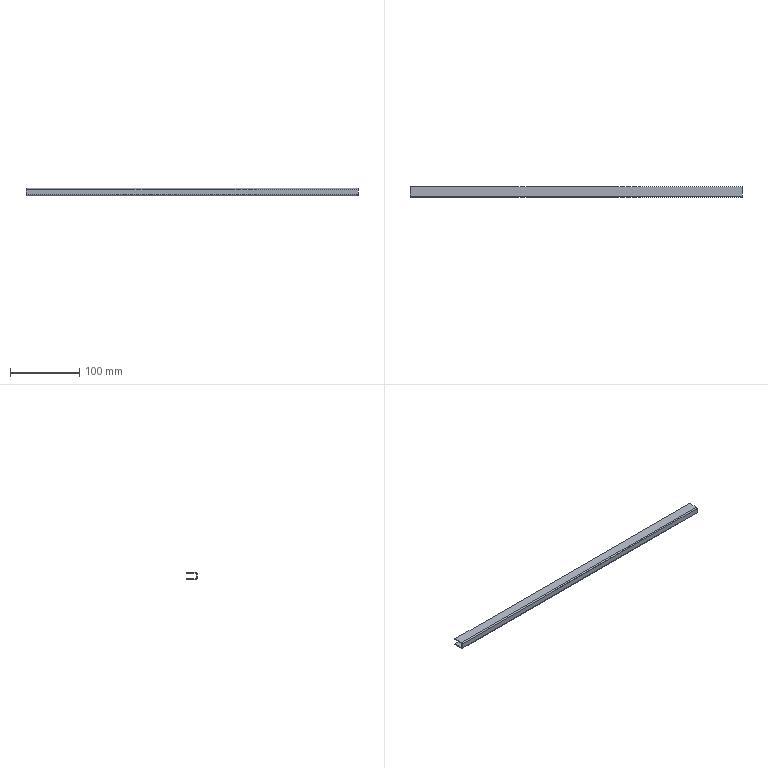Part | SolidWorks | features EdgeFlange 1, FlatPattern 1, SMBaseFlange 1, SheetMetal 1 | 1 solid | 22 faces | box 480 x 15 x 10.4 mm | volume 21369 mm3 | plane 18 | cylinder 4 | commonest cylinder face diameters 0.9 x2 3.3 x2
STEP:
#1=CARTESIAN_POINT('',(-74.374,1.2,10.26));
#2=VERTEX_POINT('',#1);
#3=CARTESIAN_POINT('',(-74.374,0.,10.26));
#4=VERTEX_POINT('',#3);
#5=CARTESIAN_POINT('',(-74.374,1.2,10.26));
#6=DIRECTION('',(0.,-1.,0.));
#7=VECTOR('',#6,1000.);
#8=LINE('',#5,#7);
#9=EDGE_CURVE('',#2,#4,#8,.T.);
#10=ORIENTED_EDGE('',*,*,#9,.F.);
#11=CARTESIAN_POINT('',(-74.374,1.2,3.16));
#12=VERTEX_POINT('',#11);
#13=CARTESIAN_POINT('',(-74.374,1.2,1.51));
#14=DIRECTION('',(0.,0.,1.));
#15=VECTOR('',#14,1000.);
#16=LINE('',#13,#15);
#17=EDGE_CURVE('',#12,#2,#16,.T.);
#18=ORIENTED_EDGE('',*,*,#17,.F.);
#19=CARTESIAN_POINT('',(-74.374,0.,3.16));
#20=VERTEX_POINT('',#19);
#21=CARTESIAN_POINT('',(-74.374,1.2,3.16));
#22=DIRECTION('',(0.,-1.,0.));
#23=VECTOR('',#22,1000.);
#24=LINE('',#21,#23);
#25=EDGE_CURVE('',#12,#20,#24,.T.);
#26=ORIENTED_EDGE('',*,*,#25,.T.);
#27=CARTESIAN_POINT('',(-74.374,0.,1.51));
#28=DIRECTION('',(0.,0.,1.));
#29=VECTOR('',#28,1000.);
#30=LINE('',#27,#29);
#31=EDGE_CURVE('',#20,#4,#30,.T.);
#32=ORIENTED_EDGE('',*,*,#31,.T.);
#33=EDGE_LOOP('',(#10,#18,#26,#32));
#34=FACE_OUTER_BOUND('',#33,.T.);
#35=CARTESIAN_POINT('',(-74.374,1.2,1.51));
#36=DIRECTION('',(1.,0.,0.));
#37=DIRECTION('',(0.,0.,-1.));
#38=AXIS2_PLACEMENT_3D('',#35,#36,#37);
#39=PLANE('',#38);
#40=ADVANCED_FACE('',(#34),#39,.F.);
#41=CARTESIAN_POINT('',(405.626,1.2,10.26));
#42=VERTEX_POINT('',#41);
#43=CARTESIAN_POINT('',(405.626,0.,10.26));
#44=VERTEX_POINT('',#43);
#45=CARTESIAN_POINT('',(405.626,1.2,10.26));
#46=DIRECTION('',(0.,-1.,0.));
#47=VECTOR('',#46,1000.);
#48=LINE('',#45,#47);
#49=EDGE_CURVE('',#42,#44,#48,.T.);
#50=ORIENTED_EDGE('',*,*,#49,.T.);
#51=CARTESIAN_POINT('',(405.626,0.,3.16));
#52=VERTEX_POINT('',#51);
#53=CARTESIAN_POINT('',(405.626,0.,1.51));
#54=DIRECTION('',(0.,0.,-1.));
#55=VECTOR('',#54,1000.);
#56=LINE('',#53,#55);
#57=EDGE_CURVE('',#44,#52,#56,.T.);
#58=ORIENTED_EDGE('',*,*,#57,.T.);
#59=CARTESIAN_POINT('',(405.626,1.2,3.16));
#60=VERTEX_POINT('',#59);
#61=CARTESIAN_POINT('',(405.626,1.2,3.16));
#62=DIRECTION('',(0.,-1.,0.));
#63=VECTOR('',#62,1000.);
#64=LINE('',#61,#63);
#65=EDGE_CURVE('',#60,#52,#64,.T.);
#66=ORIENTED_EDGE('',*,*,#65,.F.);
#67=CARTESIAN_POINT('',(405.626,1.2,1.51));
#68=DIRECTION('',(0.,0.,-1.));
#69=VECTOR('',#68,1000.);
#70=LINE('',#67,#69);
#71=EDGE_CURVE('',#42,#60,#70,.T.);
#72=ORIENTED_EDGE('',*,*,#71,.F.);
#73=EDGE_LOOP('',(#50,#58,#66,#72));
#74=FACE_OUTER_BOUND('',#73,.T.);
#75=CARTESIAN_POINT('',(405.626,1.2,1.51));
#76=DIRECTION('',(-1.,0.,0.));
#77=DIRECTION('',(0.,0.,1.));
#78=AXIS2_PLACEMENT_3D('',#75,#76,#77);
#79=PLANE('',#78);
#80=ADVANCED_FACE('',(#74),#79,.F.);
#81=ORIENTED_EDGE('',*,*,#17,.T.);
#82=CARTESIAN_POINT('',(405.626,1.2,10.26));
#83=DIRECTION('',(-1.,0.,0.));
#84=VECTOR('',#83,1000.);
#85=LINE('',#82,#84);
#86=EDGE_CURVE('',#42,#2,#85,.T.);
#87=ORIENTED_EDGE('',*,*,#86,.F.);
#88=ORIENTED_EDGE('',*,*,#71,.T.);
#89=CARTESIAN_POINT('',(-74.374,1.2,3.16));
#90=DIRECTION('',(1.,0.,0.));
#91=VECTOR('',#90,1000.);
#92=LINE('',#89,#91);
#93=EDGE_CURVE('',#12,#60,#92,.T.);
#94=ORIENTED_EDGE('',*,*,#93,.F.);
#95=EDGE_LOOP('',(#81,#87,#88,#94));
#96=FACE_OUTER_BOUND('',#95,.T.);
#97=CARTESIAN_POINT('',(-74.374,1.2,11.91));
#98=DIRECTION('',(0.,1.,0.));
#99=DIRECTION('',(0.,0.,1.));
#100=AXIS2_PLACEMENT_3D('',#97,#98,#99);
#101=PLANE('',#100);
#102=ADVANCED_FACE('',(#96),#101,.T.);
#103=CARTESIAN_POINT('',(405.626,0.,10.26));
#104=DIRECTION('',(-1.,0.,0.));
#105=VECTOR('',#104,1000.);
#106=LINE('',#103,#105);
#107=EDGE_CURVE('',#44,#4,#106,.T.);
#108=ORIENTED_EDGE('',*,*,#107,.T.);
#109=ORIENTED_EDGE('',*,*,#31,.F.);
#110=CARTESIAN_POINT('',(-74.374,0.,3.16));
#111=DIRECTION('',(1.,0.,0.));
#112=VECTOR('',#111,1000.);
#113=LINE('',#110,#112);
#114=EDGE_CURVE('',#20,#52,#113,.T.);
#115=ORIENTED_EDGE('',*,*,#114,.T.);
#116=ORIENTED_EDGE('',*,*,#57,.F.);
#117=EDGE_LOOP('',(#108,#109,#115,#116));
#118=FACE_OUTER_BOUND('',#117,.T.);
#119=CARTESIAN_POINT('',(-74.374,0.,11.91));
#120=DIRECTION('',(0.,1.,0.));
#121=DIRECTION('',(0.,0.,1.));
#122=AXIS2_PLACEMENT_3D('',#119,#120,#121);
#123=PLANE('',#122);
#124=ADVANCED_FACE('',(#118),#123,.F.);
#125=CARTESIAN_POINT('',(405.626,1.65,2.71));
#126=VERTEX_POINT('',#125);
#127=CARTESIAN_POINT('',(405.626,1.65,1.51));
#128=VERTEX_POINT('',#127);
#129=CARTESIAN_POINT('',(405.626,1.65,1.51));
#130=DIRECTION('',(0.,0.,-1.));
#131=VECTOR('',#130,1000.);
#132=LINE('',#129,#131);
#133=EDGE_CURVE('',#126,#128,#132,.T.);
#134=ORIENTED_EDGE('',*,*,#133,.F.);
#135=CARTESIAN_POINT('',(405.626,1.65,3.16));
#136=DIRECTION('',(1.,0.,0.));
#137=DIRECTION('',(0.,-1.,0.));
#138=AXIS2_PLACEMENT_3D('',#135,#136,#137);
#139=CIRCLE('',#138,0.45);
#140=EDGE_CURVE('',#60,#126,#139,.T.);
#141=ORIENTED_EDGE('',*,*,#140,.F.);
#142=ORIENTED_EDGE('',*,*,#65,.T.);
#143=CARTESIAN_POINT('',(405.626,1.65,3.16));
#144=DIRECTION('',(1.,0.,0.));
#145=DIRECTION('',(0.,-1.,0.));
#146=AXIS2_PLACEMENT_3D('',#143,#144,#145);
#147=CIRCLE('',#146,1.65);
#148=EDGE_CURVE('',#52,#128,#147,.T.);
#149=ORIENTED_EDGE('',*,*,#148,.T.);
#150=EDGE_LOOP('',(#134,#141,#142,#149));
#151=FACE_OUTER_BOUND('',#150,.T.);
#152=CARTESIAN_POINT('',(405.626,1.65,3.16));
#153=DIRECTION('',(1.,0.,0.));
#154=DIRECTION('',(0.,1.,0.));
#155=AXIS2_PLACEMENT_3D('',#152,#153,#154);
#156=PLANE('',#155);
#157=ADVANCED_FACE('',(#151),#156,.T.);
#158=ORIENTED_EDGE('',*,*,#114,.F.);
#159=CARTESIAN_POINT('',(-74.374,1.65,1.51));
#160=VERTEX_POINT('',#159);
#161=CARTESIAN_POINT('',(-74.374,1.65,3.16));
#162=DIRECTION('',(-1.,0.,0.));
#163=DIRECTION('',(0.,-1.,0.));
#164=AXIS2_PLACEMENT_3D('',#161,#162,#163);
#165=CIRCLE('',#164,1.65);
#166=EDGE_CURVE('',#160,#20,#165,.T.);
#167=ORIENTED_EDGE('',*,*,#166,.F.);
#168=CARTESIAN_POINT('',(405.626,1.65,1.51));
#169=DIRECTION('',(1.,0.,0.));
#170=VECTOR('',#169,1000.);
#171=LINE('',#168,#170);
#172=EDGE_CURVE('',#160,#128,#171,.T.);
#173=ORIENTED_EDGE('',*,*,#172,.T.);
#174=ORIENTED_EDGE('',*,*,#148,.F.);
#175=EDGE_LOOP('',(#158,#167,#173,#174));
#176=FACE_OUTER_BOUND('',#175,.T.);
#177=CARTESIAN_POINT('',(-74.374,1.65,3.16));
#178=DIRECTION('',(-1.,0.,0.));
#179=DIRECTION('',(0.,0.,-1.));
#180=AXIS2_PLACEMENT_3D('',#177,#178,#179);
#181=CYLINDRICAL_SURFACE('',#180,1.65);
#182=ADVANCED_FACE('',(#176),#181,.T.);
#183=CARTESIAN_POINT('',(-74.374,1.65,2.71));
#184=VERTEX_POINT('',#183);
#185=CARTESIAN_POINT('',(-74.374,1.65,3.16));
#186=DIRECTION('',(-1.,0.,0.));
#187=DIRECTION('',(0.,-1.,0.));
#188=AXIS2_PLACEMENT_3D('',#185,#186,#187);
#189=CIRCLE('',#188,0.45);
#190=EDGE_CURVE('',#184,#12,#189,.T.);
#191=ORIENTED_EDGE('',*,*,#190,.F.);
#192=CARTESIAN_POINT('',(-74.374,1.65,2.71));
#193=DIRECTION('',(0.,0.,-1.));
#194=VECTOR('',#193,1000.);
#195=LINE('',#192,#194);
#196=EDGE_CURVE('',#184,#160,#195,.T.);
#197=ORIENTED_EDGE('',*,*,#196,.T.);
#198=ORIENTED_EDGE('',*,*,#166,.T.);
#199=ORIENTED_EDGE('',*,*,#25,.F.);
#200=EDGE_LOOP('',(#191,#197,#198,#199));
#201=FACE_OUTER_BOUND('',#200,.T.);
#202=CARTESIAN_POINT('',(-74.374,1.65,3.16));
#203=DIRECTION('',(1.,0.,0.));
#204=DIRECTION('',(0.,1.,0.));
#205=AXIS2_PLACEMENT_3D('',#202,#203,#204);
#206=PLANE('',#205);
#207=ADVANCED_FACE('',(#201),#206,.F.);
#208=ORIENTED_EDGE('',*,*,#93,.T.);
#209=ORIENTED_EDGE('',*,*,#140,.T.);
#210=CARTESIAN_POINT('',(405.626,1.65,2.71));
#211=DIRECTION('',(-1.,0.,0.));
#212=VECTOR('',#211,1000.);
#213=LINE('',#210,#212);
#214=EDGE_CURVE('',#126,#184,#213,.T.);
#215=ORIENTED_EDGE('',*,*,#214,.T.);
#216=ORIENTED_EDGE('',*,*,#190,.T.);
#217=EDGE_LOOP('',(#208,#209,#215,#216));
#218=FACE_OUTER_BOUND('',#217,.T.);
#219=CARTESIAN_POINT('',(-74.374,1.65,3.16));
#220=DIRECTION('',(-1.,0.,0.));
#221=DIRECTION('',(0.,0.,-1.));
#222=AXIS2_PLACEMENT_3D('',#219,#220,#221);
#223=CYLINDRICAL_SURFACE('',#222,0.45);
#224=ADVANCED_FACE('',(#218),#223,.F.);
#225=ORIENTED_EDGE('',*,*,#133,.T.);
#226=CARTESIAN_POINT('',(405.626,15.,1.51));
#227=VERTEX_POINT('',#226);
#228=CARTESIAN_POINT('',(405.626,15.,1.51));
#229=DIRECTION('',(0.,-1.,0.));
#230=VECTOR('',#229,1000.);
#231=LINE('',#228,#230);
#232=EDGE_CURVE('',#227,#128,#231,.T.);
#233=ORIENTED_EDGE('',*,*,#232,.F.);
#234=CARTESIAN_POINT('',(405.626,15.,2.71));
#235=VERTEX_POINT('',#234);
#236=CARTESIAN_POINT('',(405.626,15.,1.51));
#237=DIRECTION('',(0.,0.,1.));
#238=VECTOR('',#237,1000.);
#239=LINE('',#236,#238);
#240=EDGE_CURVE('',#227,#235,#239,.T.);
#241=ORIENTED_EDGE('',*,*,#240,.T.);
#242=CARTESIAN_POINT('',(405.626,1.2,2.71));
#243=DIRECTION('',(0.,-1.,0.));
#244=VECTOR('',#243,1000.);
#245=LINE('',#242,#244);
#246=EDGE_CURVE('',#235,#126,#245,.T.);
#247=ORIENTED_EDGE('',*,*,#246,.T.);
#248=EDGE_LOOP('',(#225,#233,#241,#247));
#249=FACE_OUTER_BOUND('',#248,.T.);
#250=CARTESIAN_POINT('',(405.626,1.2,1.51));
#251=DIRECTION('',(-1.,0.,0.));
#252=DIRECTION('',(0.,0.,1.));
#253=AXIS2_PLACEMENT_3D('',#250,#251,#252);
#254=PLANE('',#253);
#255=ADVANCED_FACE('',(#249),#254,.F.);
#256=ORIENTED_EDGE('',*,*,#196,.F.);
#257=CARTESIAN_POINT('',(-74.374,15.,2.71));
#258=VERTEX_POINT('',#257);
#259=CARTESIAN_POINT('',(-74.374,15.,2.71));
#260=DIRECTION('',(0.,1.,0.));
#261=VECTOR('',#260,1000.);
#262=LINE('',#259,#261);
#263=EDGE_CURVE('',#184,#258,#262,.T.);
#264=ORIENTED_EDGE('',*,*,#263,.T.);
#265=CARTESIAN_POINT('',(-74.374,15.,1.51));
#266=VERTEX_POINT('',#265);
#267=CARTESIAN_POINT('',(-74.374,15.,1.51));
#268=DIRECTION('',(0.,0.,1.));
#269=VECTOR('',#268,1000.);
#270=LINE('',#267,#269);
#271=EDGE_CURVE('',#266,#258,#270,.T.);
#272=ORIENTED_EDGE('',*,*,#271,.F.);
#273=CARTESIAN_POINT('',(-74.374,15.,1.51));
#274=DIRECTION('',(0.,1.,0.));
#275=VECTOR('',#274,1000.);
#276=LINE('',#273,#275);
#277=EDGE_CURVE('',#160,#266,#276,.T.);
#278=ORIENTED_EDGE('',*,*,#277,.F.);
#279=EDGE_LOOP('',(#256,#264,#272,#278));
#280=FACE_OUTER_BOUND('',#279,.T.);
#281=CARTESIAN_POINT('',(-74.374,15.,1.51));
#282=DIRECTION('',(1.,0.,0.));
#283=DIRECTION('',(0.,0.,-1.));
#284=AXIS2_PLACEMENT_3D('',#281,#282,#283);
#285=PLANE('',#284);
#286=ADVANCED_FACE('',(#280),#285,.F.);
#287=ORIENTED_EDGE('',*,*,#172,.F.);
#288=ORIENTED_EDGE('',*,*,#277,.T.);
#289=CARTESIAN_POINT('',(405.626,15.,1.51));
#290=DIRECTION('',(1.,0.,0.));
#291=VECTOR('',#290,1000.);
#292=LINE('',#289,#291);
#293=EDGE_CURVE('',#266,#227,#292,.T.);
#294=ORIENTED_EDGE('',*,*,#293,.T.);
#295=ORIENTED_EDGE('',*,*,#232,.T.);
#296=EDGE_LOOP('',(#287,#288,#294,#295));
#297=FACE_OUTER_BOUND('',#296,.T.);
#298=CARTESIAN_POINT('',(405.626,15.,1.51));
#299=DIRECTION('',(0.,0.,1.));
#300=DIRECTION('',(0.,-1.,0.));
#301=AXIS2_PLACEMENT_3D('',#298,#299,#300);
#302=PLANE('',#301);
#303=ADVANCED_FACE('',(#297),#302,.F.);
#304=ORIENTED_EDGE('',*,*,#263,.F.);
#305=ORIENTED_EDGE('',*,*,#214,.F.);
#306=ORIENTED_EDGE('',*,*,#246,.F.);
#307=CARTESIAN_POINT('',(405.626,15.,2.71));
#308=DIRECTION('',(1.,0.,0.));
#309=VECTOR('',#308,1000.);
#310=LINE('',#307,#309);
#311=EDGE_CURVE('',#258,#235,#310,.T.);
#312=ORIENTED_EDGE('',*,*,#311,.F.);
#313=EDGE_LOOP('',(#304,#305,#306,#312));
#314=FACE_OUTER_BOUND('',#313,.T.);
#315=CARTESIAN_POINT('',(405.626,15.,2.71));
#316=DIRECTION('',(0.,0.,1.));
#317=DIRECTION('',(0.,-1.,0.));
#318=AXIS2_PLACEMENT_3D('',#315,#316,#317);
#319=PLANE('',#318);
#320=ADVANCED_FACE('',(#314),#319,.T.);
#321=ORIENTED_EDGE('',*,*,#311,.T.);
#322=ORIENTED_EDGE('',*,*,#240,.F.);
#323=ORIENTED_EDGE('',*,*,#293,.F.);
#324=ORIENTED_EDGE('',*,*,#271,.T.);
#325=EDGE_LOOP('',(#321,#322,#323,#324));
#326=FACE_OUTER_BOUND('',#325,.T.);
#327=CARTESIAN_POINT('',(405.626,15.,1.51));
#328=DIRECTION('',(0.,-1.,0.));
#329=DIRECTION('',(0.,0.,-1.));
#330=AXIS2_PLACEMENT_3D('',#327,#328,#329);
#331=PLANE('',#330);
#332=ADVANCED_FACE('',(#326),#331,.F.);
#333=CARTESIAN_POINT('',(-74.374,1.65,10.71));
#334=VERTEX_POINT('',#333);
#335=CARTESIAN_POINT('',(-74.374,1.65,11.91));
#336=VERTEX_POINT('',#335);
#337=CARTESIAN_POINT('',(-74.374,1.65,11.91));
#338=DIRECTION('',(0.,0.,1.));
#339=VECTOR('',#338,1000.);
#340=LINE('',#337,#339);
#341=EDGE_CURVE('',#334,#336,#340,.T.);
#342=ORIENTED_EDGE('',*,*,#341,.F.);
#343=CARTESIAN_POINT('',(-74.374,1.65,10.26));
#344=DIRECTION('',(-1.,0.,0.));
#345=DIRECTION('',(0.,0.,-1.));
#346=AXIS2_PLACEMENT_3D('',#343,#344,#345);
#347=CIRCLE('',#346,0.45);
#348=EDGE_CURVE('',#2,#334,#347,.T.);
#349=ORIENTED_EDGE('',*,*,#348,.F.);
#350=ORIENTED_EDGE('',*,*,#9,.T.);
#351=CARTESIAN_POINT('',(-74.374,1.65,10.26));
#352=DIRECTION('',(-1.,0.,0.));
#353=DIRECTION('',(0.,0.,-1.));
#354=AXIS2_PLACEMENT_3D('',#351,#352,#353);
#355=CIRCLE('',#354,1.65);
#356=EDGE_CURVE('',#4,#336,#355,.T.);
#357=ORIENTED_EDGE('',*,*,#356,.T.);
#358=EDGE_LOOP('',(#342,#349,#350,#357));
#359=FACE_OUTER_BOUND('',#358,.T.);
#360=CARTESIAN_POINT('',(-74.374,1.65,10.26));
#361=DIRECTION('',(-1.,0.,0.));
#362=DIRECTION('',(0.,0.,1.));
#363=AXIS2_PLACEMENT_3D('',#360,#361,#362);
#364=PLANE('',#363);
#365=ADVANCED_FACE('',(#359),#364,.T.);
#366=ORIENTED_EDGE('',*,*,#107,.F.);
#367=CARTESIAN_POINT('',(405.626,1.65,11.91));
#368=VERTEX_POINT('',#367);
#369=CARTESIAN_POINT('',(405.626,1.65,10.26));
#370=DIRECTION('',(1.,0.,0.));
#371=DIRECTION('',(0.,0.,-1.));
#372=AXIS2_PLACEMENT_3D('',#369,#370,#371);
#373=CIRCLE('',#372,1.65);
#374=EDGE_CURVE('',#368,#44,#373,.T.);
#375=ORIENTED_EDGE('',*,*,#374,.F.);
#376=CARTESIAN_POINT('',(-74.374,1.65,11.91));
#377=DIRECTION('',(-1.,0.,0.));
#378=VECTOR('',#377,1000.);
#379=LINE('',#376,#378);
#380=EDGE_CURVE('',#368,#336,#379,.T.);
#381=ORIENTED_EDGE('',*,*,#380,.T.);
#382=ORIENTED_EDGE('',*,*,#356,.F.);
#383=EDGE_LOOP('',(#366,#375,#381,#382));
#384=FACE_OUTER_BOUND('',#383,.T.);
#385=CARTESIAN_POINT('',(405.626,1.65,10.26));
#386=DIRECTION('',(1.,0.,0.));
#387=DIRECTION('',(0.,0.,1.));
#388=AXIS2_PLACEMENT_3D('',#385,#386,#387);
#389=CYLINDRICAL_SURFACE('',#388,1.65);
#390=ADVANCED_FACE('',(#384),#389,.T.);
#391=CARTESIAN_POINT('',(405.626,1.65,10.71));
#392=VERTEX_POINT('',#391);
#393=CARTESIAN_POINT('',(405.626,1.65,10.26));
#394=DIRECTION('',(1.,0.,0.));
#395=DIRECTION('',(0.,0.,-1.));
#396=AXIS2_PLACEMENT_3D('',#393,#394,#395);
#397=CIRCLE('',#396,0.45);
#398=EDGE_CURVE('',#392,#42,#397,.T.);
#399=ORIENTED_EDGE('',*,*,#398,.F.);
#400=CARTESIAN_POINT('',(405.626,1.65,10.71));
#401=DIRECTION('',(0.,0.,1.));
#402=VECTOR('',#401,1000.);
#403=LINE('',#400,#402);
#404=EDGE_CURVE('',#392,#368,#403,.T.);
#405=ORIENTED_EDGE('',*,*,#404,.T.);
#406=ORIENTED_EDGE('',*,*,#374,.T.);
#407=ORIENTED_EDGE('',*,*,#49,.F.);
#408=EDGE_LOOP('',(#399,#405,#406,#407));
#409=FACE_OUTER_BOUND('',#408,.T.);
#410=CARTESIAN_POINT('',(405.626,1.65,10.26));
#411=DIRECTION('',(-1.,0.,0.));
#412=DIRECTION('',(0.,0.,1.));
#413=AXIS2_PLACEMENT_3D('',#410,#411,#412);
#414=PLANE('',#413);
#415=ADVANCED_FACE('',(#409),#414,.F.);
#416=ORIENTED_EDGE('',*,*,#86,.T.);
#417=ORIENTED_EDGE('',*,*,#348,.T.);
#418=CARTESIAN_POINT('',(-74.374,1.65,10.71));
#419=DIRECTION('',(1.,0.,0.));
#420=VECTOR('',#419,1000.);
#421=LINE('',#418,#420);
#422=EDGE_CURVE('',#334,#392,#421,.T.);
#423=ORIENTED_EDGE('',*,*,#422,.T.);
#424=ORIENTED_EDGE('',*,*,#398,.T.);
#425=EDGE_LOOP('',(#416,#417,#423,#424));
#426=FACE_OUTER_BOUND('',#425,.T.);
#427=CARTESIAN_POINT('',(405.626,1.65,10.26));
#428=DIRECTION('',(1.,0.,0.));
#429=DIRECTION('',(0.,0.,1.));
#430=AXIS2_PLACEMENT_3D('',#427,#428,#429);
#431=CYLINDRICAL_SURFACE('',#430,0.45);
#432=ADVANCED_FACE('',(#426),#431,.F.);
#433=ORIENTED_EDGE('',*,*,#341,.T.);
#434=CARTESIAN_POINT('',(-74.374,15.,11.91));
#435=VERTEX_POINT('',#434);
#436=CARTESIAN_POINT('',(-74.374,15.,11.91));
#437=DIRECTION('',(0.,-1.,0.));
#438=VECTOR('',#437,1000.);
#439=LINE('',#436,#438);
#440=EDGE_CURVE('',#435,#336,#439,.T.);
#441=ORIENTED_EDGE('',*,*,#440,.F.);
#442=CARTESIAN_POINT('',(-74.374,15.,10.71));
#443=VERTEX_POINT('',#442);
#444=CARTESIAN_POINT('',(-74.374,15.,11.91));
#445=DIRECTION('',(0.,0.,-1.));
#446=VECTOR('',#445,1000.);
#447=LINE('',#444,#446);
#448=EDGE_CURVE('',#435,#443,#447,.T.);
#449=ORIENTED_EDGE('',*,*,#448,.T.);
#450=CARTESIAN_POINT('',(-74.374,1.2,10.71));
#451=DIRECTION('',(0.,-1.,0.));
#452=VECTOR('',#451,1000.);
#453=LINE('',#450,#452);
#454=EDGE_CURVE('',#443,#334,#453,.T.);
#455=ORIENTED_EDGE('',*,*,#454,.T.);
#456=EDGE_LOOP('',(#433,#441,#449,#455));
#457=FACE_OUTER_BOUND('',#456,.T.);
#458=CARTESIAN_POINT('',(-74.374,1.2,11.91));
#459=DIRECTION('',(1.,0.,0.));
#460=DIRECTION('',(0.,0.,-1.));
#461=AXIS2_PLACEMENT_3D('',#458,#459,#460);
#462=PLANE('',#461);
#463=ADVANCED_FACE('',(#457),#462,.F.);
#464=ORIENTED_EDGE('',*,*,#404,.F.);
#465=CARTESIAN_POINT('',(405.626,15.,10.71));
#466=VERTEX_POINT('',#465);
#467=CARTESIAN_POINT('',(405.626,15.,10.71));
#468=DIRECTION('',(0.,1.,0.));
#469=VECTOR('',#468,1000.);
#470=LINE('',#467,#469);
#471=EDGE_CURVE('',#392,#466,#470,.T.);
#472=ORIENTED_EDGE('',*,*,#471,.T.);
#473=CARTESIAN_POINT('',(405.626,15.,11.91));
#474=VERTEX_POINT('',#473);
#475=CARTESIAN_POINT('',(405.626,15.,11.91));
#476=DIRECTION('',(0.,0.,-1.));
#477=VECTOR('',#476,1000.);
#478=LINE('',#475,#477);
#479=EDGE_CURVE('',#474,#466,#478,.T.);
#480=ORIENTED_EDGE('',*,*,#479,.F.);
#481=CARTESIAN_POINT('',(405.626,15.,11.91));
#482=DIRECTION('',(0.,1.,0.));
#483=VECTOR('',#482,1000.);
#484=LINE('',#481,#483);
#485=EDGE_CURVE('',#368,#474,#484,.T.);
#486=ORIENTED_EDGE('',*,*,#485,.F.);
#487=EDGE_LOOP('',(#464,#472,#480,#486));
#488=FACE_OUTER_BOUND('',#487,.T.);
#489=CARTESIAN_POINT('',(405.626,15.,11.91));
#490=DIRECTION('',(-1.,0.,0.));
#491=DIRECTION('',(0.,0.,1.));
#492=AXIS2_PLACEMENT_3D('',#489,#490,#491);
#493=PLANE('',#492);
#494=ADVANCED_FACE('',(#488),#493,.F.);
#495=ORIENTED_EDGE('',*,*,#380,.F.);
#496=ORIENTED_EDGE('',*,*,#485,.T.);
#497=CARTESIAN_POINT('',(-74.374,15.,11.91));
#498=DIRECTION('',(-1.,0.,0.));
#499=VECTOR('',#498,1000.);
#500=LINE('',#497,#499);
#501=EDGE_CURVE('',#474,#435,#500,.T.);
#502=ORIENTED_EDGE('',*,*,#501,.T.);
#503=ORIENTED_EDGE('',*,*,#440,.T.);
#504=EDGE_LOOP('',(#495,#496,#502,#503));
#505=FACE_OUTER_BOUND('',#504,.T.);
#506=CARTESIAN_POINT('',(-74.374,15.,11.91));
#507=DIRECTION('',(0.,0.,-1.));
#508=DIRECTION('',(-1.,0.,0.));
#509=AXIS2_PLACEMENT_3D('',#506,#507,#508);
#510=PLANE('',#509);
#511=ADVANCED_FACE('',(#505),#510,.F.);
#512=ORIENTED_EDGE('',*,*,#471,.F.);
#513=ORIENTED_EDGE('',*,*,#422,.F.);
#514=ORIENTED_EDGE('',*,*,#454,.F.);
#515=CARTESIAN_POINT('',(-74.374,15.,10.71));
#516=DIRECTION('',(-1.,0.,0.));
#517=VECTOR('',#516,1000.);
#518=LINE('',#515,#517);
#519=EDGE_CURVE('',#466,#443,#518,.T.);
#520=ORIENTED_EDGE('',*,*,#519,.F.);
#521=EDGE_LOOP('',(#512,#513,#514,#520));
#522=FACE_OUTER_BOUND('',#521,.T.);
#523=CARTESIAN_POINT('',(-74.374,15.,10.71));
#524=DIRECTION('',(0.,0.,-1.));
#525=DIRECTION('',(-1.,0.,0.));
#526=AXIS2_PLACEMENT_3D('',#523,#524,#525);
#527=PLANE('',#526);
#528=ADVANCED_FACE('',(#522),#527,.T.);
#529=ORIENTED_EDGE('',*,*,#519,.T.);
#530=ORIENTED_EDGE('',*,*,#448,.F.);
#531=ORIENTED_EDGE('',*,*,#501,.F.);
#532=ORIENTED_EDGE('',*,*,#479,.T.);
#533=EDGE_LOOP('',(#529,#530,#531,#532));
#534=FACE_OUTER_BOUND('',#533,.T.);
#535=CARTESIAN_POINT('',(-74.374,15.,11.91));
#536=DIRECTION('',(0.,-1.,0.));
#537=DIRECTION('',(0.,0.,-1.));
#538=AXIS2_PLACEMENT_3D('',#535,#536,#537);
#539=PLANE('',#538);
#540=ADVANCED_FACE('',(#534),#539,.F.);
#541=CLOSED_SHELL('',(#40,#80,#102,#124,#157,#182,#207,#224,#255,#286,#303,#320,#332,#365,#390,#415,#432,#463,#494,#511,#528,#540));
#542=MANIFOLD_SOLID_BREP('',#541);
#543=CARTESIAN_POINT('',(0.,0.,0.));
#544=DIRECTION('',(0.,0.,1.));
#545=DIRECTION('',(1.,0.,0.));
#546=AXIS2_PLACEMENT_3D('',#543,#544,#545);
#547=(LENGTH_UNIT()NAMED_UNIT(*)SI_UNIT(.MILLI.,.METRE.));
#548=UNCERTAINTY_MEASURE_WITH_UNIT(LENGTH_MEASURE(0.00001),#547,'','');
#549=(NAMED_UNIT(*)PLANE_ANGLE_UNIT()SI_UNIT($,.RADIAN.));
#550=(NAMED_UNIT(*)SI_UNIT($,.STERADIAN.)SOLID_ANGLE_UNIT());
#551=(GEOMETRIC_REPRESENTATION_CONTEXT(3)GLOBAL_UNCERTAINTY_ASSIGNED_CONTEXT((#548))GLOBAL_UNIT_ASSIGNED_CONTEXT((#547,#549,#550))REPRESENTATION_CONTEXT('',''));
#552=ADVANCED_BREP_SHAPE_REPRESENTATION('',(#542,#546),#551);